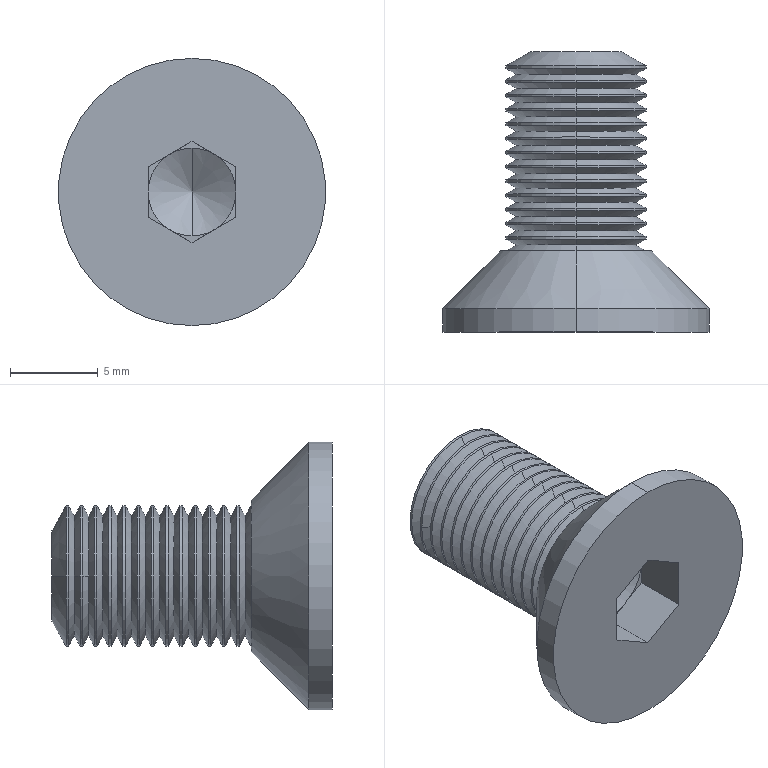Part | SolidWorks | features BaseBody 1 | 1 solid | 101 faces | box 15.24 x 16 x 15.24 mm | volume 1046 mm3 | cone 58 | cylinder 28 | plane 15 | commonest cylinder face diameters 8 x26 15.24 x2